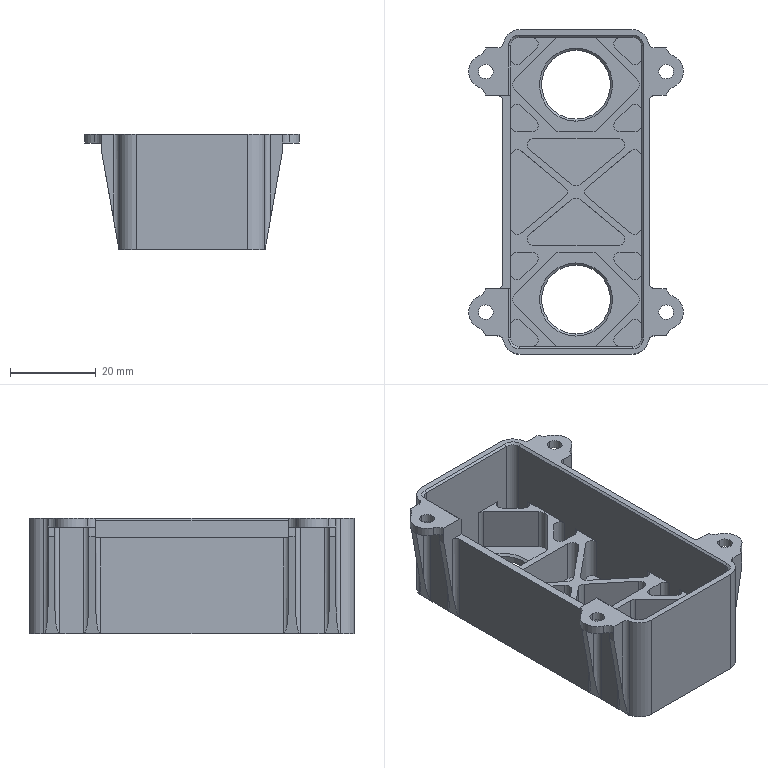Part | 1 solid | 203 faces | box 50 x 75.58 x 26.8 mm | volume 18797 mm3 | plane 103 | cylinder 92 | cone 8 | commonest cylinder face diameters 3 x40 2.5 x16 3.4 x8 4 x8 6 x8 8 x8